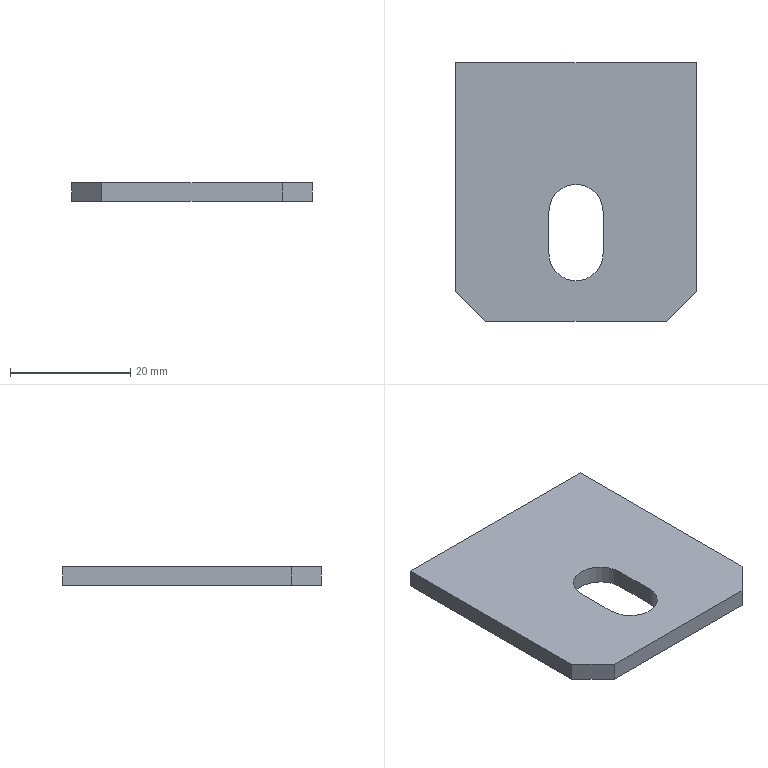Part | SolidWorks | features Extrusion 1 | 1 solid | 12 faces | box 40 x 43 x 3 mm | volume 4705 mm3 | plane 10 | cylinder 2 | commonest cylinder face diameters 9 x2
STEP:
#1=CARTESIAN_POINT('',(213.585,213.495,3.));
#2=VERTEX_POINT('',#1);
#3=CARTESIAN_POINT('',(213.585,175.495,3.));
#4=VERTEX_POINT('',#3);
#5=CARTESIAN_POINT('',(213.585,175.495,3.));
#6=DIRECTION('',(0.,-1.,0.));
#7=VECTOR('',#6,1000.);
#8=LINE('',#5,#7);
#9=EDGE_CURVE('',#2,#4,#8,.T.);
#10=ORIENTED_EDGE('',*,*,#9,.T.);
#11=CARTESIAN_POINT('',(218.585,170.495,3.));
#12=VERTEX_POINT('',#11);
#13=CARTESIAN_POINT('',(218.585,170.495,3.));
#14=DIRECTION('',(0.7071,-0.7071,0.));
#15=VECTOR('',#14,1000.);
#16=LINE('',#13,#15);
#17=EDGE_CURVE('',#4,#12,#16,.T.);
#18=ORIENTED_EDGE('',*,*,#17,.T.);
#19=CARTESIAN_POINT('',(248.585,170.495,3.));
#20=VERTEX_POINT('',#19);
#21=CARTESIAN_POINT('',(248.585,170.495,3.));
#22=DIRECTION('',(1.,0.,0.));
#23=VECTOR('',#22,1000.);
#24=LINE('',#21,#23);
#25=EDGE_CURVE('',#12,#20,#24,.T.);
#26=ORIENTED_EDGE('',*,*,#25,.T.);
#27=CARTESIAN_POINT('',(253.585,175.495,3.));
#28=VERTEX_POINT('',#27);
#29=CARTESIAN_POINT('',(248.585,170.495,3.));
#30=DIRECTION('',(0.7071,0.7071,0.));
#31=VECTOR('',#30,1000.);
#32=LINE('',#29,#31);
#33=EDGE_CURVE('',#20,#28,#32,.T.);
#34=ORIENTED_EDGE('',*,*,#33,.T.);
#35=CARTESIAN_POINT('',(253.585,213.495,3.));
#36=VERTEX_POINT('',#35);
#37=CARTESIAN_POINT('',(253.585,213.495,3.));
#38=DIRECTION('',(0.,1.,0.));
#39=VECTOR('',#38,1000.);
#40=LINE('',#37,#39);
#41=EDGE_CURVE('',#28,#36,#40,.T.);
#42=ORIENTED_EDGE('',*,*,#41,.T.);
#43=CARTESIAN_POINT('',(213.585,213.495,3.));
#44=DIRECTION('',(-1.,0.,0.));
#45=VECTOR('',#44,1000.);
#46=LINE('',#43,#45);
#47=EDGE_CURVE('',#36,#2,#46,.T.);
#48=ORIENTED_EDGE('',*,*,#47,.T.);
#49=EDGE_LOOP('',(#10,#18,#26,#34,#42,#48));
#50=FACE_OUTER_BOUND('',#49,.T.);
#51=CARTESIAN_POINT('',(229.085,181.745,3.));
#52=VERTEX_POINT('',#51);
#53=CARTESIAN_POINT('',(238.085,181.745,3.));
#54=VERTEX_POINT('',#53);
#55=CARTESIAN_POINT('',(233.585,181.745,3.));
#56=DIRECTION('',(0.,0.,1.));
#57=DIRECTION('',(1.,0.,0.));
#58=AXIS2_PLACEMENT_3D('',#55,#56,#57);
#59=CIRCLE('',#58,4.5);
#60=EDGE_CURVE('',#52,#54,#59,.T.);
#61=ORIENTED_EDGE('',*,*,#60,.F.);
#62=CARTESIAN_POINT('',(229.085,188.745,3.));
#63=VERTEX_POINT('',#62);
#64=CARTESIAN_POINT('',(229.085,181.745,3.));
#65=DIRECTION('',(0.,-1.,0.));
#66=VECTOR('',#65,1000.);
#67=LINE('',#64,#66);
#68=EDGE_CURVE('',#63,#52,#67,.T.);
#69=ORIENTED_EDGE('',*,*,#68,.F.);
#70=CARTESIAN_POINT('',(238.085,188.745,3.));
#71=VERTEX_POINT('',#70);
#72=CARTESIAN_POINT('',(233.585,188.745,3.));
#73=DIRECTION('',(0.,0.,1.));
#74=DIRECTION('',(1.,0.,0.));
#75=AXIS2_PLACEMENT_3D('',#72,#73,#74);
#76=CIRCLE('',#75,4.5);
#77=EDGE_CURVE('',#71,#63,#76,.T.);
#78=ORIENTED_EDGE('',*,*,#77,.F.);
#79=CARTESIAN_POINT('',(238.085,181.745,3.));
#80=DIRECTION('',(0.,1.,0.));
#81=VECTOR('',#80,1000.);
#82=LINE('',#79,#81);
#83=EDGE_CURVE('',#54,#71,#82,.T.);
#84=ORIENTED_EDGE('',*,*,#83,.F.);
#85=EDGE_LOOP('',(#61,#69,#78,#84));
#86=FACE_BOUND('',#85,.T.);
#87=CARTESIAN_POINT('',(0.,0.,3.));
#88=DIRECTION('',(0.,0.,-1.));
#89=DIRECTION('',(-1.,0.,0.));
#90=AXIS2_PLACEMENT_3D('',#87,#88,#89);
#91=PLANE('',#90);
#92=ADVANCED_FACE('',(#50,#86),#91,.F.);
#93=CARTESIAN_POINT('',(213.585,213.495,0.));
#94=VERTEX_POINT('',#93);
#95=CARTESIAN_POINT('',(213.585,175.495,0.));
#96=VERTEX_POINT('',#95);
#97=CARTESIAN_POINT('',(213.585,175.495,0.));
#98=DIRECTION('',(0.,-1.,0.));
#99=VECTOR('',#98,1000.);
#100=LINE('',#97,#99);
#101=EDGE_CURVE('',#94,#96,#100,.T.);
#102=ORIENTED_EDGE('',*,*,#101,.F.);
#103=CARTESIAN_POINT('',(253.585,213.495,0.));
#104=VERTEX_POINT('',#103);
#105=CARTESIAN_POINT('',(213.585,213.495,0.));
#106=DIRECTION('',(-1.,0.,0.));
#107=VECTOR('',#106,1000.);
#108=LINE('',#105,#107);
#109=EDGE_CURVE('',#104,#94,#108,.T.);
#110=ORIENTED_EDGE('',*,*,#109,.F.);
#111=CARTESIAN_POINT('',(253.585,175.495,0.));
#112=VERTEX_POINT('',#111);
#113=CARTESIAN_POINT('',(253.585,213.495,0.));
#114=DIRECTION('',(0.,1.,0.));
#115=VECTOR('',#114,1000.);
#116=LINE('',#113,#115);
#117=EDGE_CURVE('',#112,#104,#116,.T.);
#118=ORIENTED_EDGE('',*,*,#117,.F.);
#119=CARTESIAN_POINT('',(248.585,170.495,0.));
#120=VERTEX_POINT('',#119);
#121=CARTESIAN_POINT('',(248.585,170.495,0.));
#122=DIRECTION('',(0.7071,0.7071,0.));
#123=VECTOR('',#122,1000.);
#124=LINE('',#121,#123);
#125=EDGE_CURVE('',#120,#112,#124,.T.);
#126=ORIENTED_EDGE('',*,*,#125,.F.);
#127=CARTESIAN_POINT('',(218.585,170.495,0.));
#128=VERTEX_POINT('',#127);
#129=CARTESIAN_POINT('',(248.585,170.495,0.));
#130=DIRECTION('',(1.,0.,0.));
#131=VECTOR('',#130,1000.);
#132=LINE('',#129,#131);
#133=EDGE_CURVE('',#128,#120,#132,.T.);
#134=ORIENTED_EDGE('',*,*,#133,.F.);
#135=CARTESIAN_POINT('',(218.585,170.495,0.));
#136=DIRECTION('',(0.7071,-0.7071,0.));
#137=VECTOR('',#136,1000.);
#138=LINE('',#135,#137);
#139=EDGE_CURVE('',#96,#128,#138,.T.);
#140=ORIENTED_EDGE('',*,*,#139,.F.);
#141=EDGE_LOOP('',(#102,#110,#118,#126,#134,#140));
#142=FACE_OUTER_BOUND('',#141,.T.);
#143=CARTESIAN_POINT('',(229.085,188.745,0.));
#144=VERTEX_POINT('',#143);
#145=CARTESIAN_POINT('',(229.085,181.745,0.));
#146=VERTEX_POINT('',#145);
#147=CARTESIAN_POINT('',(229.085,181.745,0.));
#148=DIRECTION('',(0.,-1.,0.));
#149=VECTOR('',#148,1000.);
#150=LINE('',#147,#149);
#151=EDGE_CURVE('',#144,#146,#150,.T.);
#152=ORIENTED_EDGE('',*,*,#151,.T.);
#153=CARTESIAN_POINT('',(238.085,181.745,0.));
#154=VERTEX_POINT('',#153);
#155=CARTESIAN_POINT('',(233.585,181.745,0.));
#156=DIRECTION('',(0.,0.,1.));
#157=DIRECTION('',(1.,0.,0.));
#158=AXIS2_PLACEMENT_3D('',#155,#156,#157);
#159=CIRCLE('',#158,4.5);
#160=EDGE_CURVE('',#146,#154,#159,.T.);
#161=ORIENTED_EDGE('',*,*,#160,.T.);
#162=CARTESIAN_POINT('',(238.085,188.745,0.));
#163=VERTEX_POINT('',#162);
#164=CARTESIAN_POINT('',(238.085,181.745,0.));
#165=DIRECTION('',(0.,1.,0.));
#166=VECTOR('',#165,1000.);
#167=LINE('',#164,#166);
#168=EDGE_CURVE('',#154,#163,#167,.T.);
#169=ORIENTED_EDGE('',*,*,#168,.T.);
#170=CARTESIAN_POINT('',(233.585,188.745,0.));
#171=DIRECTION('',(0.,0.,1.));
#172=DIRECTION('',(1.,0.,0.));
#173=AXIS2_PLACEMENT_3D('',#170,#171,#172);
#174=CIRCLE('',#173,4.5);
#175=EDGE_CURVE('',#163,#144,#174,.T.);
#176=ORIENTED_EDGE('',*,*,#175,.T.);
#177=EDGE_LOOP('',(#152,#161,#169,#176));
#178=FACE_BOUND('',#177,.T.);
#179=CARTESIAN_POINT('',(0.,0.,0.));
#180=DIRECTION('',(0.,0.,-1.));
#181=DIRECTION('',(-1.,0.,0.));
#182=AXIS2_PLACEMENT_3D('',#179,#180,#181);
#183=PLANE('',#182);
#184=ADVANCED_FACE('',(#142,#178),#183,.T.);
#185=ORIENTED_EDGE('',*,*,#101,.T.);
#186=CARTESIAN_POINT('',(213.585,175.495,3.));
#187=DIRECTION('',(0.,0.,-1.));
#188=VECTOR('',#187,1000.);
#189=LINE('',#186,#188);
#190=EDGE_CURVE('',#4,#96,#189,.T.);
#191=ORIENTED_EDGE('',*,*,#190,.F.);
#192=ORIENTED_EDGE('',*,*,#9,.F.);
#193=CARTESIAN_POINT('',(213.585,213.495,3.));
#194=DIRECTION('',(0.,0.,-1.));
#195=VECTOR('',#194,1000.);
#196=LINE('',#193,#195);
#197=EDGE_CURVE('',#2,#94,#196,.T.);
#198=ORIENTED_EDGE('',*,*,#197,.T.);
#199=EDGE_LOOP('',(#185,#191,#192,#198));
#200=FACE_OUTER_BOUND('',#199,.T.);
#201=CARTESIAN_POINT('',(213.585,175.495,3.));
#202=DIRECTION('',(1.,0.,0.));
#203=DIRECTION('',(0.,1.,0.));
#204=AXIS2_PLACEMENT_3D('',#201,#202,#203);
#205=PLANE('',#204);
#206=ADVANCED_FACE('',(#200),#205,.F.);
#207=ORIENTED_EDGE('',*,*,#139,.T.);
#208=CARTESIAN_POINT('',(218.585,170.495,3.));
#209=DIRECTION('',(0.,0.,-1.));
#210=VECTOR('',#209,1000.);
#211=LINE('',#208,#210);
#212=EDGE_CURVE('',#12,#128,#211,.T.);
#213=ORIENTED_EDGE('',*,*,#212,.F.);
#214=ORIENTED_EDGE('',*,*,#17,.F.);
#215=ORIENTED_EDGE('',*,*,#190,.T.);
#216=EDGE_LOOP('',(#207,#213,#214,#215));
#217=FACE_OUTER_BOUND('',#216,.T.);
#218=CARTESIAN_POINT('',(218.585,170.495,3.));
#219=DIRECTION('',(0.7071,0.7071,0.));
#220=DIRECTION('',(-0.7071,0.7071,0.));
#221=AXIS2_PLACEMENT_3D('',#218,#219,#220);
#222=PLANE('',#221);
#223=ADVANCED_FACE('',(#217),#222,.F.);
#224=ORIENTED_EDGE('',*,*,#133,.T.);
#225=CARTESIAN_POINT('',(248.585,170.495,3.));
#226=DIRECTION('',(0.,0.,-1.));
#227=VECTOR('',#226,1000.);
#228=LINE('',#225,#227);
#229=EDGE_CURVE('',#20,#120,#228,.T.);
#230=ORIENTED_EDGE('',*,*,#229,.F.);
#231=ORIENTED_EDGE('',*,*,#25,.F.);
#232=ORIENTED_EDGE('',*,*,#212,.T.);
#233=EDGE_LOOP('',(#224,#230,#231,#232));
#234=FACE_OUTER_BOUND('',#233,.T.);
#235=CARTESIAN_POINT('',(248.585,170.495,3.));
#236=DIRECTION('',(0.,1.,0.));
#237=DIRECTION('',(-1.,0.,0.));
#238=AXIS2_PLACEMENT_3D('',#235,#236,#237);
#239=PLANE('',#238);
#240=ADVANCED_FACE('',(#234),#239,.F.);
#241=ORIENTED_EDGE('',*,*,#125,.T.);
#242=CARTESIAN_POINT('',(253.585,175.495,3.));
#243=DIRECTION('',(0.,0.,-1.));
#244=VECTOR('',#243,1000.);
#245=LINE('',#242,#244);
#246=EDGE_CURVE('',#28,#112,#245,.T.);
#247=ORIENTED_EDGE('',*,*,#246,.F.);
#248=ORIENTED_EDGE('',*,*,#33,.F.);
#249=ORIENTED_EDGE('',*,*,#229,.T.);
#250=EDGE_LOOP('',(#241,#247,#248,#249));
#251=FACE_OUTER_BOUND('',#250,.T.);
#252=CARTESIAN_POINT('',(248.585,170.495,3.));
#253=DIRECTION('',(-0.7071,0.7071,0.));
#254=DIRECTION('',(-0.7071,-0.7071,0.));
#255=AXIS2_PLACEMENT_3D('',#252,#253,#254);
#256=PLANE('',#255);
#257=ADVANCED_FACE('',(#251),#256,.F.);
#258=ORIENTED_EDGE('',*,*,#117,.T.);
#259=CARTESIAN_POINT('',(253.585,213.495,3.));
#260=DIRECTION('',(0.,0.,-1.));
#261=VECTOR('',#260,1000.);
#262=LINE('',#259,#261);
#263=EDGE_CURVE('',#36,#104,#262,.T.);
#264=ORIENTED_EDGE('',*,*,#263,.F.);
#265=ORIENTED_EDGE('',*,*,#41,.F.);
#266=ORIENTED_EDGE('',*,*,#246,.T.);
#267=EDGE_LOOP('',(#258,#264,#265,#266));
#268=FACE_OUTER_BOUND('',#267,.T.);
#269=CARTESIAN_POINT('',(253.585,213.495,3.));
#270=DIRECTION('',(-1.,0.,0.));
#271=DIRECTION('',(0.,0.,1.));
#272=AXIS2_PLACEMENT_3D('',#269,#270,#271);
#273=PLANE('',#272);
#274=ADVANCED_FACE('',(#268),#273,.F.);
#275=ORIENTED_EDGE('',*,*,#109,.T.);
#276=ORIENTED_EDGE('',*,*,#197,.F.);
#277=ORIENTED_EDGE('',*,*,#47,.F.);
#278=ORIENTED_EDGE('',*,*,#263,.T.);
#279=EDGE_LOOP('',(#275,#276,#277,#278));
#280=FACE_OUTER_BOUND('',#279,.T.);
#281=CARTESIAN_POINT('',(213.585,213.495,3.));
#282=DIRECTION('',(0.,-1.,0.));
#283=DIRECTION('',(0.,0.,-1.));
#284=AXIS2_PLACEMENT_3D('',#281,#282,#283);
#285=PLANE('',#284);
#286=ADVANCED_FACE('',(#280),#285,.F.);
#287=ORIENTED_EDGE('',*,*,#160,.F.);
#288=CARTESIAN_POINT('',(229.085,181.745,3.));
#289=DIRECTION('',(0.,0.,-1.));
#290=VECTOR('',#289,1000.);
#291=LINE('',#288,#290);
#292=EDGE_CURVE('',#52,#146,#291,.T.);
#293=ORIENTED_EDGE('',*,*,#292,.F.);
#294=ORIENTED_EDGE('',*,*,#60,.T.);
#295=CARTESIAN_POINT('',(238.085,181.745,3.));
#296=DIRECTION('',(0.,0.,-1.));
#297=VECTOR('',#296,1000.);
#298=LINE('',#295,#297);
#299=EDGE_CURVE('',#54,#154,#298,.T.);
#300=ORIENTED_EDGE('',*,*,#299,.T.);
#301=EDGE_LOOP('',(#287,#293,#294,#300));
#302=FACE_OUTER_BOUND('',#301,.T.);
#303=CARTESIAN_POINT('',(233.585,181.745,3.));
#304=DIRECTION('',(0.,0.,-1.));
#305=DIRECTION('',(-1.,0.,0.));
#306=AXIS2_PLACEMENT_3D('',#303,#304,#305);
#307=CYLINDRICAL_SURFACE('',#306,4.5);
#308=ADVANCED_FACE('',(#302),#307,.F.);
#309=ORIENTED_EDGE('',*,*,#168,.F.);
#310=ORIENTED_EDGE('',*,*,#299,.F.);
#311=ORIENTED_EDGE('',*,*,#83,.T.);
#312=CARTESIAN_POINT('',(238.085,188.745,3.));
#313=DIRECTION('',(0.,0.,-1.));
#314=VECTOR('',#313,1000.);
#315=LINE('',#312,#314);
#316=EDGE_CURVE('',#71,#163,#315,.T.);
#317=ORIENTED_EDGE('',*,*,#316,.T.);
#318=EDGE_LOOP('',(#309,#310,#311,#317));
#319=FACE_OUTER_BOUND('',#318,.T.);
#320=CARTESIAN_POINT('',(238.085,181.745,3.));
#321=DIRECTION('',(-1.,0.,0.));
#322=DIRECTION('',(0.,0.,1.));
#323=AXIS2_PLACEMENT_3D('',#320,#321,#322);
#324=PLANE('',#323);
#325=ADVANCED_FACE('',(#319),#324,.T.);
#326=ORIENTED_EDGE('',*,*,#175,.F.);
#327=ORIENTED_EDGE('',*,*,#316,.F.);
#328=ORIENTED_EDGE('',*,*,#77,.T.);
#329=CARTESIAN_POINT('',(229.085,188.745,3.));
#330=DIRECTION('',(0.,0.,-1.));
#331=VECTOR('',#330,1000.);
#332=LINE('',#329,#331);
#333=EDGE_CURVE('',#63,#144,#332,.T.);
#334=ORIENTED_EDGE('',*,*,#333,.T.);
#335=EDGE_LOOP('',(#326,#327,#328,#334));
#336=FACE_OUTER_BOUND('',#335,.T.);
#337=CARTESIAN_POINT('',(233.585,188.745,3.));
#338=DIRECTION('',(0.,0.,-1.));
#339=DIRECTION('',(-1.,0.,0.));
#340=AXIS2_PLACEMENT_3D('',#337,#338,#339);
#341=CYLINDRICAL_SURFACE('',#340,4.5);
#342=ADVANCED_FACE('',(#336),#341,.F.);
#343=ORIENTED_EDGE('',*,*,#151,.F.);
#344=ORIENTED_EDGE('',*,*,#333,.F.);
#345=ORIENTED_EDGE('',*,*,#68,.T.);
#346=ORIENTED_EDGE('',*,*,#292,.T.);
#347=EDGE_LOOP('',(#343,#344,#345,#346));
#348=FACE_OUTER_BOUND('',#347,.T.);
#349=CARTESIAN_POINT('',(229.085,181.745,3.));
#350=DIRECTION('',(1.,0.,0.));
#351=DIRECTION('',(0.,0.,-1.));
#352=AXIS2_PLACEMENT_3D('',#349,#350,#351);
#353=PLANE('',#352);
#354=ADVANCED_FACE('',(#348),#353,.T.);
#355=CLOSED_SHELL('',(#92,#184,#206,#223,#240,#257,#274,#286,#308,#325,#342,#354));
#356=MANIFOLD_SOLID_BREP('',#355);
#357=CARTESIAN_POINT('',(0.,0.,0.));
#358=DIRECTION('',(0.,0.,1.));
#359=DIRECTION('',(1.,0.,0.));
#360=AXIS2_PLACEMENT_3D('',#357,#358,#359);
#361=(LENGTH_UNIT()NAMED_UNIT(*)SI_UNIT(.MILLI.,.METRE.));
#362=UNCERTAINTY_MEASURE_WITH_UNIT(LENGTH_MEASURE(0.00001),#361,'','');
#363=(NAMED_UNIT(*)PLANE_ANGLE_UNIT()SI_UNIT($,.RADIAN.));
#364=(NAMED_UNIT(*)SI_UNIT($,.STERADIAN.)SOLID_ANGLE_UNIT());
#365=(GEOMETRIC_REPRESENTATION_CONTEXT(3)GLOBAL_UNCERTAINTY_ASSIGNED_CONTEXT((#362))GLOBAL_UNIT_ASSIGNED_CONTEXT((#361,#363,#364))REPRESENTATION_CONTEXT('',''));
#366=ADVANCED_BREP_SHAPE_REPRESENTATION('',(#356,#360),#365);